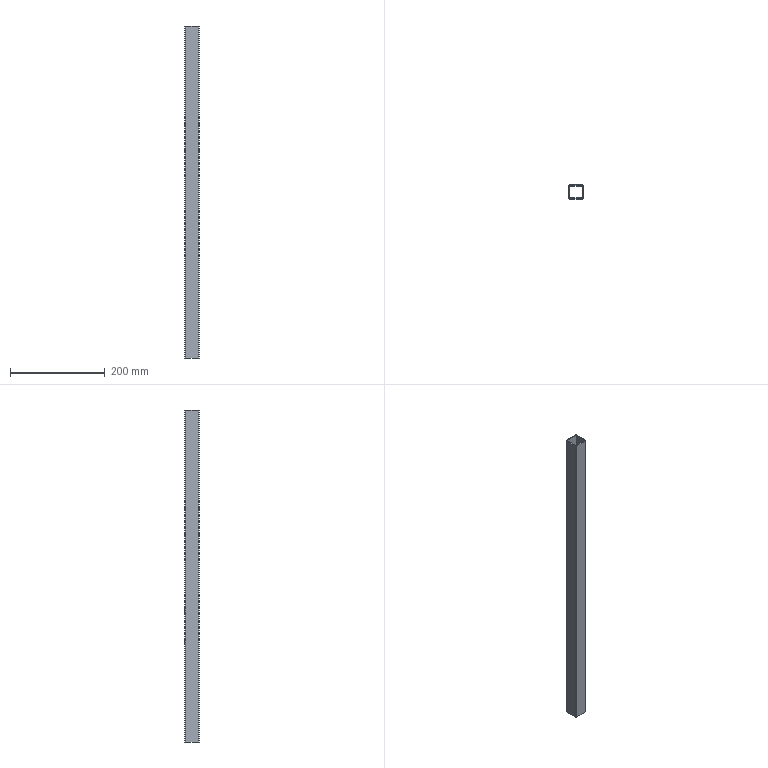Part | STEP file | Q7C1206 | 1 solid | 18 faces | box 30 x 30 x 700 mm | volume 154296 mm3 | plane 10 | cylinder 8 | commonest cylinder face diameters 4 x8